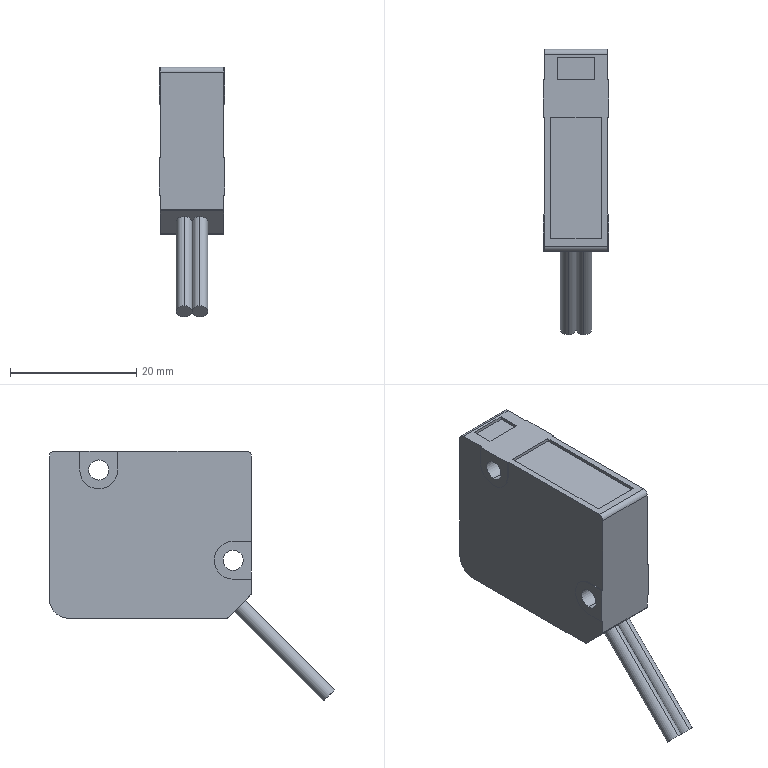Part | STEP file | Proximity Switch | 1 solid | 49 faces | box 10.4 x 45.161 x 39.591 mm | volume 8353 mm3 | plane 30 | cylinder 19 | commonest cylinder face diameters 2.5 x6 6 x5 3.2 x4 0.6 x2 1.6 x2